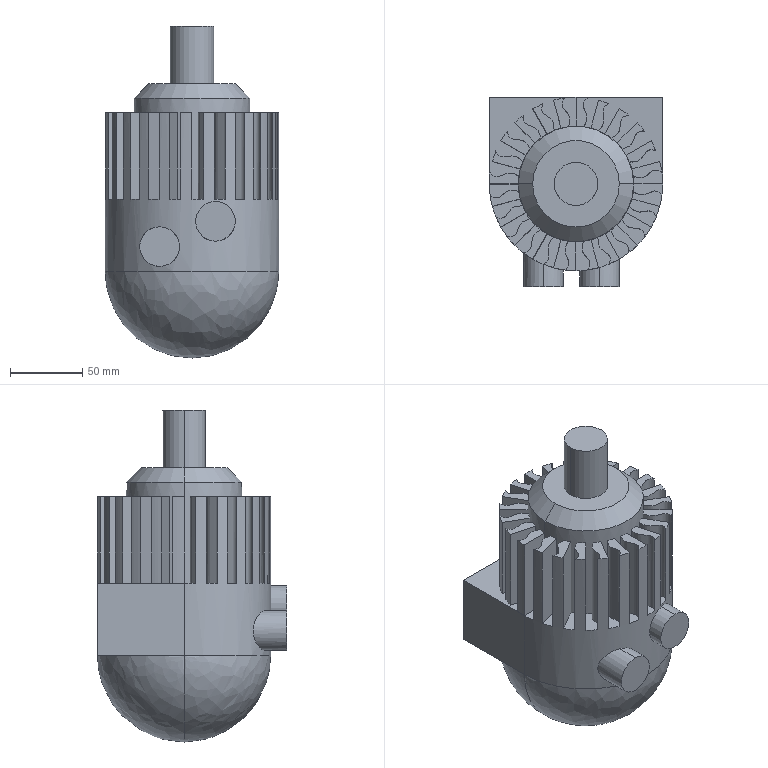Part | SolidWorks | features BaseBody 1, ICE 1 | 1 solid | 144 faces | box 120 x 131 x 230 mm | volume 1709728 mm3 | plane 71 | cylinder 29 | spline 26 | cone 18 | commonest cylinder face diameters 120 x13 8.5 x8 27.442 x4 30 x2 80 x2